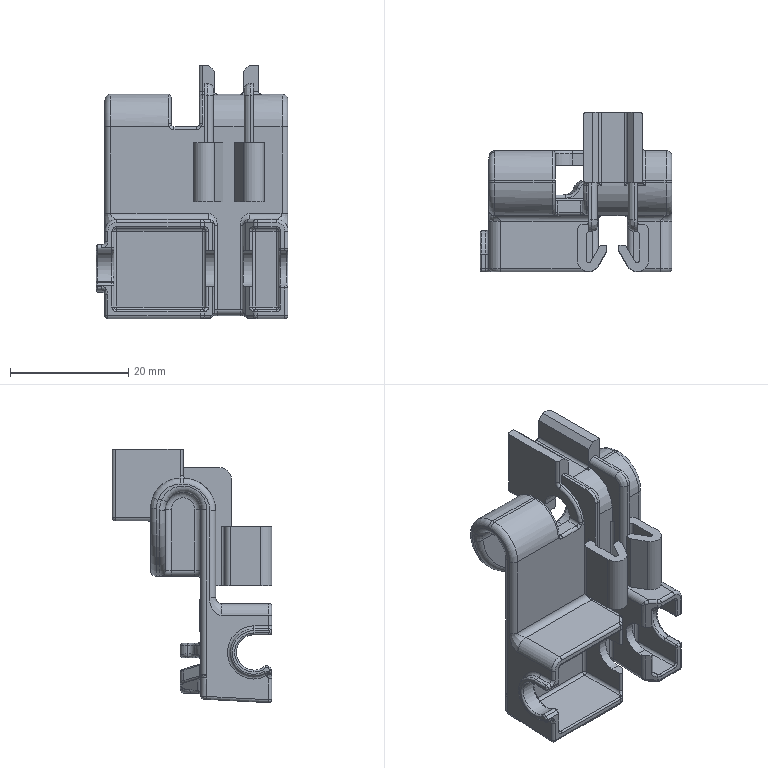Part | STEP file | ZXW735-L-232_2_1_1 | 1 solid | 475 faces | box 32.5 x 27 x 42.902 mm | volume 6709 mm3 | cylinder 197 | plane 133 | torus 63 | spline 61 | sphere 21 | commonest cylinder face diameters 1 x96 2 x34 0.6 x28 6 x10 3.6 x6 4 x6